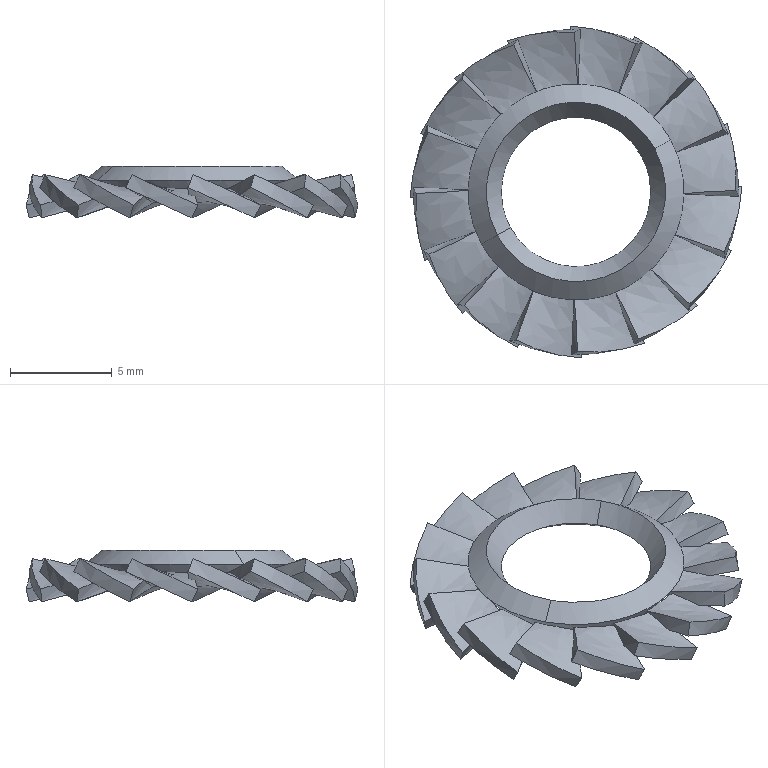Part | NX | features BREP 1 | 1 solid | 104 faces | box 16.312 x 16.312 x 2.545 mm | volume 132.852 mm3 | spline 96 | cone 8